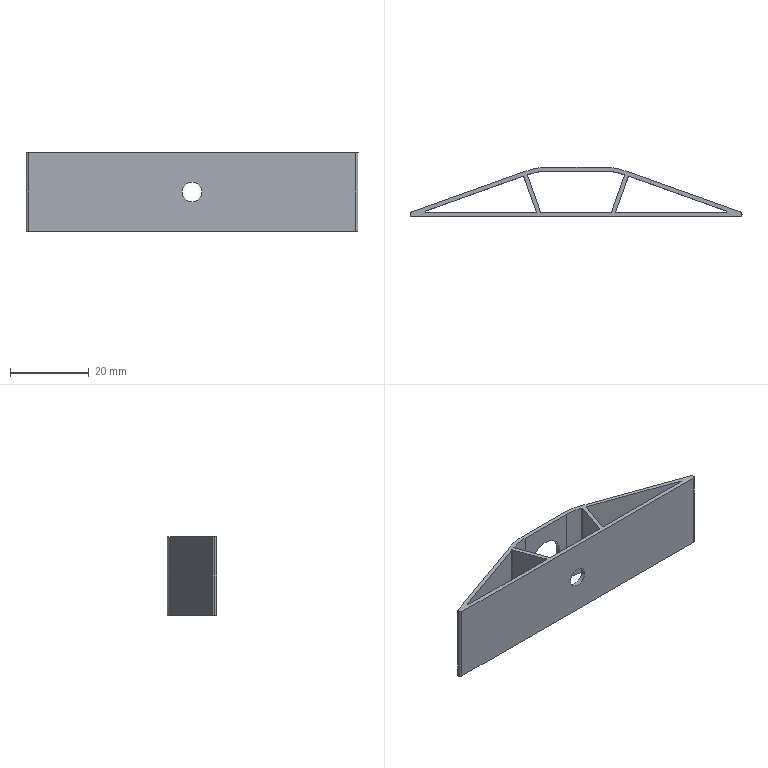Part | STEP file | V00-000000449 | 1 solid | 46 faces | box 84.272 x 12.5 x 20 mm | volume 3695 mm3 | cylinder 28 | plane 18 | commonest cylinder face diameters 0.4 x16 1.2 x4 5 x2 10 x2 28 x2 30 x2